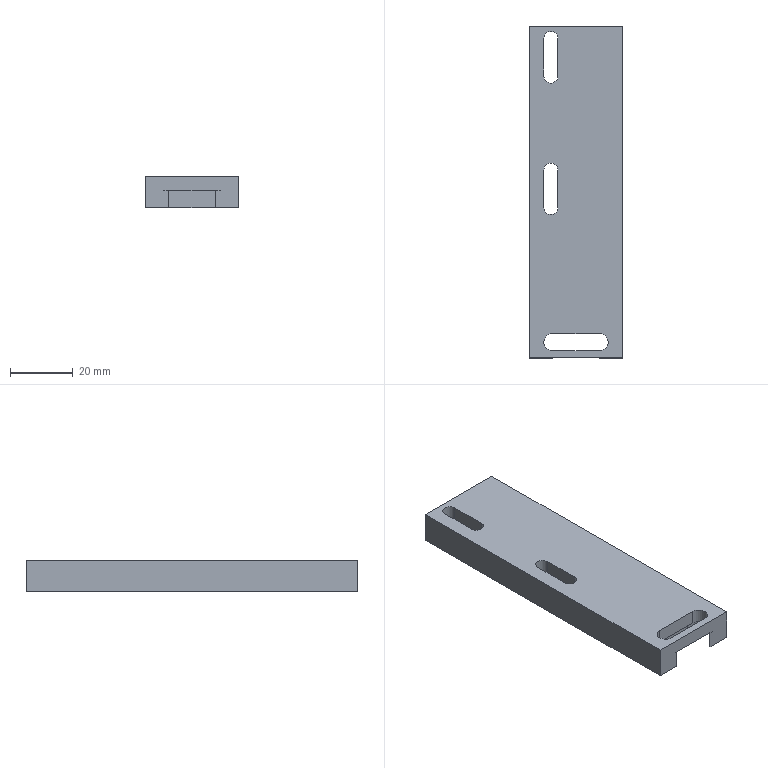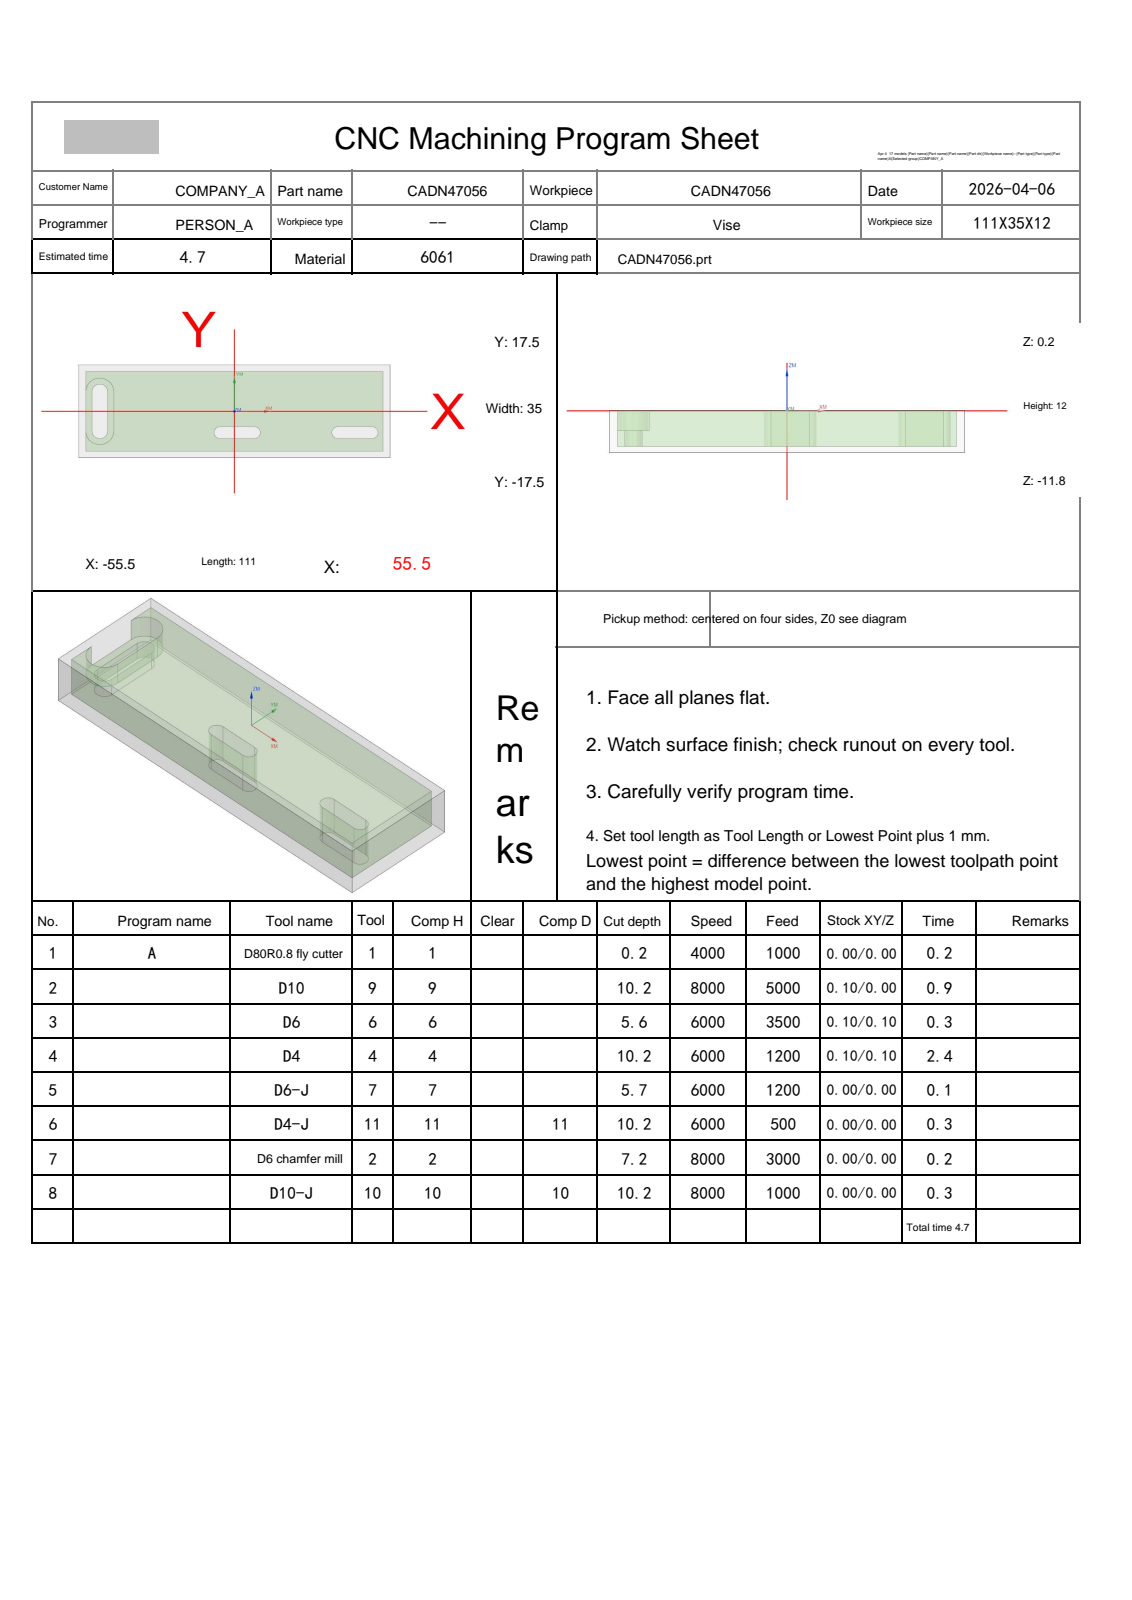NC program | NX | posted by the shop | part box 30 x 106 x 10 mm
Whole program:
%
O0001
(Machine time: 6.39 MIN)
(===Total Tool:8===)
(T1=D80R0.8 fly cutter D=80.  R=0.8  D-  H01 Z=0.    )
(T9=D10     D=10.  R=0.   D-  H09 Z=-10.  )
(T6=D6      D=6.   R=0.   D-  H06 Z=-5.4  )
(T4=D4      D=4.   R=0.   D-  H04 Z=-10.  )
(T7=D6-J    D=6.   R=0.   D7  H07 Z=-5.5  )
(T11=D4-J   D=4.   R=0.   D11 H11 Z=-10.  )
(T2=D6 chamfer mill   D=6.   R=0.   D-  H02 Z=-7.   )
(T10=D10-J  D=10.  R=0.   D10 H10 Z=-10.  )
G80 G90 G17 G49 G40
G91 G28 Z0
M01
N1 T01 M06
(D80R0.8 fly cutter  D=80. R=0.8 H=01 ce=0.00 di=0.00)
G00 G90 G54 X-98. Y0.0 M03 S4000
G43 H01 Z20.
M08
Z2.
G01 Z0.0 F1000.
X-93.
X93.
X98.
Z2.
G00 Z20.
G91 G28 Z0.0
M05
M09
G91 G28 Z0.0
M01
N2 T09 M06
(D10  D=10. R=0. H=09 ce=0.10 di=0.00)
G00 G90 G54 X0.0 Y20.1 M03 S8000
G43 H09 Z20.
M08
Z.5
G01 X53. Z.369 F5000.
G02 X58.1 Y15. Z.35 I0.0 J-5.1
G01 Y-15. Z.275
G02 X53. Y-20.1 Z.256 I-5.1 J0.0
G01 X-53. Z-.006
G02 X-58.1 Y-15. Z-.025 I0.0 J5.1
G01 Y15. Z-.1
G02 X-53. Y20.1 Z-.119 I5.1 J0.0
G01 X53. Z-.381
G02 X58.1 Y15. Z-.4 I0.0 J-5.1
G01 Y-15. Z-.475
G02 X53. Y-20.1 Z-.494 I-5.1 J0.0
G01 X-53. Z-.756
G02 X-58.1 Y-15. Z-.775 I0.0 J5.1
G01 Y15. Z-.85
G02 X-53. Y20.1 Z-.869 I5.1 J0.0
G01 X53. Z-1.131
G02 X58.1 Y15. Z-1.15 I0.0 J-5.1
G01 Y-15. Z-1.225
G02 X53. Y-20.1 Z-1.244 I-5.1 J0.0
G01 X-53. Z-1.506
G02 X-58.1 Y-15. Z-1.525 I0.0 J5.1
G01 Y15. Z-1.6
G02 X-53. Y20.1 Z-1.619 I5.1 J0.0
G01 X53. Z-1.881
G02 X58.1 Y15. Z-1.9 I0.0 J-5.1
G01 Y-15. Z-1.975
G02 X53. Y-20.1 Z-1.994 I-5.1 J0.0
G01 X-53. Z-2.256
G02 X-58.1 Y-15. Z-2.275 I0.0 J5.1
G01 Y15. Z-2.35
G02 X-53. Y20.1 Z-2.369 I5.1 J0.0
G01 X53. Z-2.631
G02 X58.1 Y15. Z-2.65 I0.0 J-5.1
G01 Y-15. Z-2.725
G02 X53. Y-20.1 Z-2.744 I-5.1 J0.0
G01 X-53. Z-3.006
G02 X-58.1 Y-15. Z-3.025 I0.0 J5.1
G01 Y15. Z-3.1
G02 X-53. Y20.1 Z-3.119 I5.1 J0.0
G01 X53. Z-3.381
G02 X58.1 Y15. Z-3.4 I0.0 J-5.1
G01 Y-15. Z-3.475
G02 X53. Y-20.1 Z-3.494 I-5.1 J0.0
G01 X-53. Z-3.756
G02 X-58.1 Y-15. Z-3.775 I0.0 J5.1
G01 Y15. Z-3.85
G02 X-53. Y20.1 Z-3.869 I5.1 J0.0
G01 X53. Z-4.131
G02 X58.1 Y15. Z-4.15 I0.0 J-5.1
G01 Y-15. Z-4.225
G02 X53. Y-20.1 Z-4.244 I-5.1 J0.0
G01 X-53. Z-4.506
G02 X-58.1 Y-15. Z-4.525 I0.0 J5.1
G01 Y15. Z-4.6
G02 X-53. Y20.1 Z-4.619 I5.1 J0.0
G01 X53. Z-4.881
G02 X58.1 Y15. Z-4.9 I0.0 J-5.1
G01 Y-15. Z-4.975
G02 X53. Y-20.1 Z-4.994 I-5.1 J0.0
G01 X-53. Z-5.256
G02 X-58.1 Y-15. Z-5.275 I0.0 J5.1
G01 Y15. Z-5.35
G02 X-53. Y20.1 Z-5.369 I5.1 J0.0
G01 X53. Z-5.631
G02 X58.1 Y15. Z-5.65 I0.0 J-5.1
G01 Y-15. Z-5.725
G02 X53. Y-20.1 Z-5.744 I-5.1 J0.0
G01 X-53. Z-6.006
G02 X-58.1 Y-15. Z-6.025 I0.0 J5.1
G01 Y15. Z-6.1
G02 X-53. Y20.1 Z-6.119 I5.1 J0.0
G01 X53. Z-6.381
G02 X58.1 Y15. Z-6.4 I0.0 J-5.1
G01 Y-15. Z-6.475
G02 X53. Y-20.1 Z-6.494 I-5.1 J0.0
G01 X-53. Z-6.756
G02 X-58.1 Y-15. Z-6.775 I0.0 J5.1
G01 Y15. Z-6.85
G02 X-53. Y20.1 Z-6.869 I5.1 J0.0
G01 X53. Z-7.131
G02 X58.1 Y15. Z-7.15 I0.0 J-5.1
G01 Y-15. Z-7.225
G02 X53. Y-20.1 Z-7.244 I-5.1 J0.0
G01 X-53. Z-7.506
G02 X-58.1 Y-15. Z-7.525 I0.0 J5.1
G01 Y15. Z-7.6
G02 X-53. Y20.1 Z-7.619 I5.1 J0.0
G01 X53. Z-7.881
G02 X58.1 Y15. Z-7.9 I0.0 J-5.1
G01 Y-15. Z-7.975
G02 X53. Y-20.1 Z-7.994 I-5.1 J0.0
G01 X-53. Z-8.256
G02 X-58.1 Y-15. Z-8.275 I0.0 J5.1
G01 Y15. Z-8.35
G02 X-53. Y20.1 Z-8.369 I5.1 J0.0
G01 X53. Z-8.631
G02 X58.1 Y15. Z-8.65 I0.0 J-5.1
G01 Y-15. Z-8.725
G02 X53. Y-20.1 Z-8.744 I-5.1 J0.0
G01 X-53. Z-9.006
G02 X-58.1 Y-15. Z-9.025 I0.0 J5.1
G01 Y15. Z-9.1
G02 X-53. Y20.1 Z-9.119 I5.1 J0.0
G01 X53. Z-9.381
G02 X58.1 Y15. Z-9.4 I0.0 J-5.1
G01 Y-15. Z-9.475
G02 X53. Y-20.1 Z-9.494 I-5.1 J0.0
G01 X-53. Z-9.756
G02 X-58.1 Y-15. Z-9.775 I0.0 J5.1
G01 Y15. Z-9.85
G02 X-53. Y20.1 Z-9.869 I5.1 J0.0
G01 X0.0 Z-10.
X53.
G02 X58.1 Y15. I0.0 J-5.1
G01 Y-15.
G02 X53. Y-20.1 I-5.1 J0.0
G01 X-53.
G02 X-58.1 Y-15. I0.0 J5.1
G01 Y15.
G02 X-53. Y20.1 I5.1 J0.0
G01 X0.0
X.5
Z-9.
G00 Z20.
G91 G28 Z0.0
M05
M09
G91 G28 Z0.0
M01
N3 T06 M06
(D6  D=6. R=0. H=06 ce=0.10 di=0.10)
G00 G90 G54 X-59. Y0.0 M03 S6000
G43 H06 Z20.
M08
Z.114
G01 Z-.386 F3500.
X-50.9
Y-2.094
G02 X-48.8 Y-3.5 I-2.1 J-5.406
G01 Y3.5
G02 X-50.9 Y2.094 I-4.2 J4.
G01 Y0.0
X-53.6
Y-4.459
G02 X-53. Y-4.4 I.6 J-3.041
X-49.9 Y-7.5 I0.0 J-3.1
G03 X-48. Y-9.4 I1.9 J0.0
X-46.1 Y-7.5 I0.0 J1.9
G01 Y7.5
G03 X-48. Y9.4 I-1.9 J0.0
X-49.9 Y7.5 I0.0 J-1.9
G02 X-53. Y4.4 I-3.1 J0.0
X-53.6 Y4.459 I0.0 J3.1
G01 Y0.0
Y-.5
Z.114
G00 Z.5
X-59. Y0.0
Z-.271
G01 Z-.771
X-50.9
Y-2.094
G02 X-48.8 Y-3.5 I-2.1 J-5.406
G01 Y3.5
G02 X-50.9 Y2.094 I-4.2 J4.
G01 Y0.0
X-53.6
Y-4.459
G02 X-53. Y-4.4 I.6 J-3.041
X-49.9 Y-7.5 I0.0 J-3.1
G03 X-48. Y-9.4 I1.9 J0.0
X-46.1 Y-7.5 I0.0 J1.9
G01 Y7.5
G03 X-48. Y9.4 I-1.9 J0.0
X-49.9 Y7.5 I0.0 J-1.9
G02 X-53. Y4.4 I-3.1 J0.0
X-53.6 Y4.459 I0.0 J3.1
G01 Y0.0
Y-.5
Z-.271
G00 Z.114
X-59. Y0.0
Z-.657
G01 Z-1.157
X-50.9
Y-2.094
G02 X-48.8 Y-3.5 I-2.1 J-5.406
G01 Y3.5
G02 X-50.9 Y2.094 I-4.2 J4.
G01 Y0.0
X-53.6
Y-4.459
G02 X-53. Y-4.4 I.6 J-3.041
X-49.9 Y-7.5 I0.0 J-3.1
G03 X-48. Y-9.4 I1.9 J0.0
X-46.1 Y-7.5 I0.0 J1.9
G01 Y7.5
G03 X-48. Y9.4 I-1.9 J0.0
X-49.9 Y7.5 I0.0 J-1.9
G02 X-53. Y4.4 I-3.1 J0.0
X-53.6 Y4.459 I0.0 J3.1
G01 Y0.0
Y-.5
Z-.657
G00 Z-.271
X-59. Y0.0
Z-1.043
G01 Z-1.543
X-50.9
Y-2.094
G02 X-48.8 Y-3.5 I-2.1 J-5.406
G01 Y3.5
G02 X-50.9 Y2.094 I-4.2 J4.
G01 Y0.0
X-53.6
Y-4.459
G02 X-53. Y-4.4 I.6 J-3.041
X-49.9 Y-7.5 I0.0 J-3.1
G03 X-48. Y-9.4 I1.9 J0.0
X-46.1 Y-7.5 I0.0 J1.9
G01 Y7.5
G03 X-48. Y9.4 I-1.9 J0.0
X-49.9 Y7.5 I0.0 J-1.9
G02 X-53. Y4.4 I-3.1 J0.0
X-53.6 Y4.459 I0.0 J3.1
G01 Y0.0
Y-.5
Z-1.043
G00 Z-.657
X-59. Y0.0
Z-1.429
G01 Z-1.929
X-50.9
Y-2.094
G02 X-48.8 Y-3.5 I-2.1 J-5.406
G01 Y3.5
G02 X-50.9 Y2.094 I-4.2 J4.
G01 Y0.0
X-53.6
Y-4.459
G02 X-53. Y-4.4 I.6 J-3.041
X-49.9 Y-7.5 I0.0 J-3.1
G03 X-48. Y-9.4 I1.9 J0.0
X-46.1 Y-7.5 I0.0 J1.9
G01 Y7.5
G03 X-48. Y9.4 I-1.9 J0.0
X-49.9 Y7.5 I0.0 J-1.9
G02 X-53. Y4.4 I-3.1 J0.0
X-53.6 Y4.459 I0.0 J3.1
G01 Y0.0
Y-.5
Z-1.429
G00 Z-1.043
X-59. Y0.0
Z-1.814
G01 Z-2.314
X-50.9
Y-2.094
G02 X-48.8 Y-3.5 I-2.1 J-5.406
G01 Y3.5
G02 X-50.9 Y2.094 I-4.2 J4.
G01 Y0.0
X-53.6
Y-4.459
G02 X-53. Y-4.4 I.6 J-3.041
X-49.9 Y-7.5 I0.0 J-3.1
G03 X-48. Y-9.4 I1.9 J0.0
X-46.1 Y-7.5 I0.0 J1.9
G01 Y7.5
G03 X-48. Y9.4 I-1.9 J0.0
X-49.9 Y7.5 I0.0 J-1.9
G02 X-53. Y4.4 I-3.1 J0.0
X-53.6 Y4.459 I0.0 J3.1
G01 Y0.0
Y-.5
Z-1.814
G00 Z-1.429
X-59. Y0.0
Z-2.2
G01 Z-2.7
X-50.9
Y-2.094
G02 X-48.8 Y-3.5 I-2.1 J-5.406
G01 Y3.5
G02 X-50.9 Y2.094 I-4.2 J4.
G01 Y0.0
X-53.6
Y-4.459
G02 X-53. Y-4.4 I.6 J-3.041
X-49.9 Y-7.5 I0.0 J-3.1
G03 X-48. Y-9.4 I1.9 J0.0
X-46.1 Y-7.5 I0.0 J1.9
G01 Y7.5
G03 X-48. Y9.4 I-1.9 J0.0
X-49.9 Y7.5 I0.0 J-1.9
G02 X-53. Y4.4 I-3.1 J0.0
X-53.6 Y4.459 I0.0 J3.1
G01 Y0.0
Y-.5
Z-2.2
G00 Z-1.814
X-59. Y0.0
Z-2.586
G01 Z-3.086
X-50.9
Y-2.094
G02 X-48.8 Y-3.5 I-2.1 J-5.406
G01 Y3.5
G02 X-50.9 Y2.094 I-4.2 J4.
G01 Y0.0
X-53.6
Y-4.459
G02 X-53. Y-4.4 I.6 J-3.041
X-49.9 Y-7.5 I0.0 J-3.1
G03 X-48. Y-9.4 I1.9 J0.0
X-46.1 Y-7.5 I0.0 J1.9
G01 Y7.5
G03 X-48. Y9.4 I-1.9 J0.0
X-49.9 Y7.5 I0.0 J-1.9
G02 X-53. Y4.4 I-3.1 J0.0
X-53.6 Y4.459 I0.0 J3.1
G01 Y0.0
Y-.5
Z-2.586
G00 Z-2.2
X-59. Y0.0
Z-2.971
G01 Z-3.471
X-50.9
Y-2.094
G02 X-48.8 Y-3.5 I-2.1 J-5.406
G01 Y3.5
G02 X-50.9 Y2.094 I-4.2 J4.
G01 Y0.0
X-53.6
Y-4.459
G02 X-53. Y-4.4 I.6 J-3.041
X-49.9 Y-7.5 I0.0 J-3.1
G03 X-48. Y-9.4 I1.9 J0.0
X-46.1 Y-7.5 I0.0 J1.9
G01 Y7.5
G03 X-48. Y9.4 I-1.9 J0.0
X-49.9 Y7.5 I0.0 J-1.9
G02 X-53. Y4.4 I-3.1 J0.0
X-53.6 Y4.459 I0.0 J3.1
G01 Y0.0
Y-.5
Z-2.971
G00 Z-2.586
X-59. Y0.0
Z-3.357
G01 Z-3.857
X-50.9
Y-2.094
G02 X-48.8 Y-3.5 I-2.1 J-5.406
G01 Y3.5
G02 X-50.9 Y2.094 I-4.2 J4.
G01 Y0.0
X-53.6
Y-4.459
G02 X-53. Y-4.4 I.6 J-3.041
X-49.9 Y-7.5 I0.0 J-3.1
G03 X-48. Y-9.4 I1.9 J0.0
X-46.1 Y-7.5 I0.0 J1.9
G01 Y7.5
G03 X-48. Y9.4 I-1.9 J0.0
X-49.9 Y7.5 I0.0 J-1.9
G02 X-53. Y4.4 I-3.1 J0.0
X-53.6 Y4.459 I0.0 J3.1
G01 Y0.0
Y-.5
Z-3.357
G00 Z-2.971
X-59. Y0.0
Z-3.743
G01 Z-4.243
X-50.9
Y-2.094
G02 X-48.8 Y-3.5 I-2.1 J-5.406
G01 Y3.5
G02 X-50.9 Y2.094 I-4.2 J4.
G01 Y0.0
X-53.6
Y-4.459
G02 X-53. Y-4.4 I.6 J-3.041
X-49.9 Y-7.5 I0.0 J-3.1
G03 X-48. Y-9.4 I1.9 J0.0
X-46.1 Y-7.5 I0.0 J1.9
G01 Y7.5
G03 X-48. Y9.4 I-1.9 J0.0
X-49.9 Y7.5 I0.0 J-1.9
G02 X-53. Y4.4 I-3.1 J0.0
X-53.6 Y4.459 I0.0 J3.1
G01 Y0.0
Y-.5
Z-3.743
G00 Z-3.357
X-59. Y0.0
Z-4.129
G01 Z-4.629
X-50.9
Y-2.094
G02 X-48.8 Y-3.5 I-2.1 J-5.406
G01 Y3.5
G02 X-50.9 Y2.094 I-4.2 J4.
G01 Y0.0
X-53.6
Y-4.459
G02 X-53. Y-4.4 I.6 J-3.041
X-49.9 Y-7.5 I0.0 J-3.1
G03 X-48. Y-9.4 I1.9 J0.0
X-46.1 Y-7.5 I0.0 J1.9
G01 Y7.5
G03 X-48. Y9.4 I-1.9 J0.0
X-49.9 Y7.5 I0.0 J-1.9
G02 X-53. Y4.4 I-3.1 J0.0
X-53.6 Y4.459 I0.0 J3.1
G01 Y0.0
Y-.5
Z-4.129
G00 Z-3.743
X-59. Y0.0
Z-4.514
G01 Z-5.014
X-50.9
Y-2.094
G02 X-48.8 Y-3.5 I-2.1 J-5.406
G01 Y3.5
G02 X-50.9 Y2.094 I-4.2 J4.
G01 Y0.0
X-53.6
Y-4.459
G02 X-53. Y-4.4 I.6 J-3.041
X-49.9 Y-7.5 I0.0 J-3.1
G03 X-48. Y-9.4 I1.9 J0.0
X-46.1 Y-7.5 I0.0 J1.9
G01 Y7.5
G03 X-48. Y9.4 I-1.9 J0.0
X-49.9 Y7.5 I0.0 J-1.9
G02 X-53. Y4.4 I-3.1 J0.0
X-53.6 Y4.459 I0.0 J3.1
G01 Y0.0
Y-.5
Z-4.514
G00 Z-4.129
X-59. Y0.0
Z-4.9
G01 Z-5.4
X-50.9
Y-2.094
G02 X-48.8 Y-3.5 I-2.1 J-5.406
G01 Y3.5
G02 X-50.9 Y2.094 I-4.2 J4.
G01 Y0.0
X-53.6
Y-4.459
G02 X-53. Y-4.4 I.6 J-3.041
X-49.9 Y-7.5 I0.0 J-3.1
G03 X-48. Y-9.4 I1.9 J0.0
X-46.1 Y-7.5 I0.0 J1.9
G01 Y7.5
G03 X-48. Y9.4 I-1.9 J0.0
X-49.9 Y7.5 I0.0 J-1.9
G02 X-53. Y4.4 I-3.1 J0.0
X-53.6 Y4.459 I0.0 J3.1
G01 Y0.0
Y-.5
Z-4.9
G00 Z20.
G91 G28 Z0.0
M05
M09
G91 G28 Z0.0
M01
N4 T04 M06
(D4  D=4. R=0. H=04 ce=0.10 di=0.10)
G00 G90 G54 X43. Y-7.85 M03 S6000
G43 H04 Z20.
M08
Z.5
G01 X37. Z.44 F1200.
G03 X36.85 Y-8. Z.438 I0.0 J-.15
X37. Y-8.15 Z.435 I.15 J0.0
G01 X49. Z.315
G03 X49.15 Y-8. Z.313 I0.0 J.15
X49. Y-7.85 Z.31 I-.15 J0.0
G01 X37. Z.19
G03 X36.85 Y-8. Z.188 I0.0 J-.15
X37. Y-8.15 Z.185 I.15 J0.0
G01 X49. Z.065
G03 X49.15 Y-8. Z.063 I0.0 J.15
X49. Y-7.85 Z.06 I-.15 J0.0
G01 X37. Z-.06
G03 X36.85 Y-8. Z-.063 I0.0 J-.15
X37. Y-8.15 Z-.065 I.15 J0.0
G01 X49. Z-.185
G03 X49.15 Y-8. Z-.188 I0.0 J.15
X49. Y-7.85 Z-.19 I-.15 J0.0
G01 X37. Z-.31
G03 X36.85 Y-8. Z-.313 I0.0 J-.15
X37. Y-8.15 Z-.315 I.15 J0.0
G01 X49. Z-.435
G03 X49.15 Y-8. Z-.438 I0.0 J.15
X49. Y-7.85 Z-.44 I-.15 J0.0
G01 X37. Z-.56
G03 X36.85 Y-8. Z-.563 I0.0 J-.15
X37. Y-8.15 Z-.565 I.15 J0.0
G01 X49. Z-.685
G03 X49.15 Y-8. Z-.688 I0.0 J.15
X49. Y-7.85 Z-.69 I-.15 J0.0
G01 X37. Z-.81
G03 X36.85 Y-8. Z-.813 I0.0 J-.15
X37. Y-8.15 Z-.815 I.15 J0.0
G01 X49. Z-.935
G03 X49.15 Y-8. Z-.938 I0.0 J.15
X49. Y-7.85 Z-.94 I-.15 J0.0
G01 X37. Z-1.06
G03 X36.85 Y-8. Z-1.063 I0.0 J-.15
X37. Y-8.15 Z-1.065 I.15 J0.0
G01 X49. Z-1.185
G03 X49.15 Y-8. Z-1.188 I0.0 J.15
X49. Y-7.85 Z-1.19 I-.15 J0.0
G01 X37. Z-1.31
G03 X36.85 Y-8. Z-1.313 I0.0 J-.15
X37. Y-8.15 Z-1.315 I.15 J0.0
G01 X49. Z-1.435
G03 X49.15 Y-8. Z-1.438 I0.0 J.15
X49. Y-7.85 Z-1.44 I-.15 J0.0
G01 X37. Z-1.56
G03 X36.85 Y-8. Z-1.563 I0.0 J-.15
X37. Y-8.15 Z-1.565 I.15 J0.0
G01 X49. Z-1.685
G03 X49.15 Y-8. Z-1.688 I0.0 J.15
X49. Y-7.85 Z-1.69 I-.15 J0.0
G01 X37. Z-1.81
G03 X36.85 Y-8. Z-1.813 I0.0 J-.15
X37. Y-8.15 Z-1.815 I.15 J0.0
G01 X49. Z-1.935
G03 X49.15 Y-8. Z-1.938 I0.0 J.15
X49. Y-7.85 Z-1.94 I-.15 J0.0
G01 X37. Z-2.06
G03 X36.85 Y-8. Z-2.063 I0.0 J-.15
X37. Y-8.15 Z-2.065 I.15 J0.0
G01 X49. Z-2.185
G03 X49.15 Y-8. Z-2.188 I0.0 J.15
X49. Y-7.85 Z-2.19 I-.15 J0.0
G01 X37. Z-2.31
G03 X36.85 Y-8. Z-2.313 I0.0 J-.15
X37. Y-8.15 Z-2.315 I.15 J0.0
G01 X49. Z-2.435
G03 X49.15 Y-8. Z-2.438 I0.0 J.15
X49. Y-7.85 Z-2.44 I-.15 J0.0
G01 X37. Z-2.56
G03 X36.85 Y-8. Z-2.563 I0.0 J-.15
X37. Y-8.15 Z-2.565 I.15 J0.0
G01 X49. Z-2.685
G03 X49.15 Y-8. Z-2.688 I0.0 J.15
X49. Y-7.85 Z-2.69 I-.15 J0.0
G01 X37. Z-2.81
G03 X36.85 Y-8. Z-2.813 I0.0 J-.15
X37. Y-8.15 Z-2.815 I.15 J0.0
G01 X49. Z-2.935
G03 X49.15 Y-8. Z-2.938 I0.0 J.15
X49. Y-7.85 Z-2.94 I-.15 J0.0
G01 X37. Z-3.06
G03 X36.85 Y-8. Z-3.063 I0.0 J-.15
X37. Y-8.15 Z-3.065 I.15 J0.0
G01 X49. Z-3.185
G03 X49.15 Y-8. Z-3.188 I0.0 J.15
X49. Y-7.85 Z-3.19 I-.15 J0.0
G01 X37. Z-3.31
G03 X36.85 Y-8. Z-3.313 I0.0 J-.15
X37. Y-8.15 Z-3.315 I.15 J0.0
G01 X49. Z-3.435
G03 X49.15 Y-8. Z-3.438 I0.0 J.15
X49. Y-7.85 Z-3.44 I-.15 J0.0
G01 X37. Z-3.56
G03 X36.85 Y-8. Z-3.563 I0.0 J-.15
X37. Y-8.15 Z-3.565 I.15 J0.0
G01 X49. Z-3.685
G03 X49.15 Y-8. Z-3.688 I0.0 J.15
X49. Y-7.85 Z-3.69 I-.15 J0.0
G01 X37. Z-3.81
G03 X36.85 Y-8. Z-3.813 I0.0 J-.15
X37. Y-8.15 Z-3.815 I.15 J0.0
G01 X49. Z-3.935
G03 X49.15 Y-8. Z-3.938 I0.0 J.15
X49. Y-7.85 Z-3.94 I-.15 J0.0
G01 X37. Z-4.06
G03 X36.85 Y-8. Z-4.063 I0.0 J-.15
X37. Y-8.15 Z-4.065 I.15 J0.0
G01 X49. Z-4.185
G03 X49.15 Y-8. Z-4.188 I0.0 J.15
X49. Y-7.85 Z-4.19 I-.15 J0.0
G01 X37. Z-4.31
G03 X36.85 Y-8. Z-4.313 I0.0 J-.15
X37. Y-8.15 Z-4.315 I.15 J0.0
G01 X49. Z-4.435
G03 X49.15 Y-8. Z-4.438 I0.0 J.15
X49. Y-7.85 Z-4.44 I-.15 J0.0
G01 X37. Z-4.56
G03 X36.85 Y-8. Z-4.563 I0.0 J-.15
X37. Y-8.15 Z-4.565 I.15 J0.0
G01 X49. Z-4.685
G03 X49.15 Y-8. Z-4.688 I0.0 J.15
X49. Y-7.85 Z-4.69 I-.15 J0.0
G01 X37. Z-4.81
G03 X36.85 Y-8. Z-4.813 I0.0 J-.15
X37. Y-8.15 Z-4.815 I.15 J0.0
G01 X49. Z-4.935
G03 X49.15 Y-8. Z-4.938 I0.0 J.15
X49. Y-7.85 Z-4.94 I-.15 J0.0
G01 X37. Z-5.06
G03 X36.85 Y-8. Z-5.063 I0.0 J-.15
X37. Y-8.15 Z-5.065 I.15 J0.0
G01 X49. Z-5.185
G03 X49.15 Y-8. Z-5.188 I0.0 J.15
X49. Y-7.85 Z-5.19 I-.15 J0.0
G01 X37. Z-5.31
G03 X36.85 Y-8. Z-5.313 I0.0 J-.15
X37. Y-8.15 Z-5.315 I.15 J0.0
G01 X49. Z-5.435
G03 X49.15 Y-8. Z-5.438 I0.0 J.15
X49. Y-7.85 Z-5.44 I-.15 J0.0
G01 X37. Z-5.56
G03 X36.85 Y-8. Z-5.563 I0.0 J-.15
X37. Y-8.15 Z-5.565 I.15 J0.0
G01 X49. Z-5.685
G03 X49.15 Y-8. Z-5.688 I0.0 J.15
X49. Y-7.85 Z-5.69 I-.15 J0.0
G01 X37. Z-5.81
G03 X36.85 Y-8. Z-5.813 I0.0 J-.15
X37. Y-8.15 Z-5.815 I.15 J0.0
G01 X49. Z-5.935
G03 X49.15 Y-8. Z-5.938 I0.0 J.15
X49. Y-7.85 Z-5.94 I-.15 J0.0
G01 X37. Z-6.06
G03 X36.85 Y-8. Z-6.063 I0.0 J-.15
X37. Y-8.15 Z-6.065 I.15 J0.0
G01 X49. Z-6.185
G03 X49.15 Y-8. Z-6.188 I0.0 J.15
X49. Y-7.85 Z-6.19 I-.15 J0.0
G01 X37. Z-6.31
G03 X36.85 Y-8. Z-6.313 I0.0 J-.15
X37. Y-8.15 Z-6.315 I.15 J0.0
G01 X49. Z-6.435
G03 X49.15 Y-8. Z-6.438 I0.0 J.15
X49. Y-7.85 Z-6.44 I-.15 J0.0
G01 X37. Z-6.56
G03 X36.85 Y-8. Z-6.563 I0.0 J-.15
X37. Y-8.15 Z-6.565 I.15 J0.0
G01 X49. Z-6.685
G03 X49.15 Y-8. Z-6.688 I0.0 J.15
X49. Y-7.85 Z-6.69 I-.15 J0.0
G01 X37. Z-6.81
G03 X36.85 Y-8. Z-6.813 I0.0 J-.15
X37. Y-8.15 Z-6.815 I.15 J0.0
G01 X49. Z-6.935
G03 X49.15 Y-8. Z-6.938 I0.0 J.15
X49. Y-7.85 Z-6.94 I-.15 J0.0
G01 X37. Z-7.06
G03 X36.85 Y-8. Z-7.063 I0.0 J-.15
X37. Y-8.15 Z-7.065 I.15 J0.0
G01 X49. Z-7.185
G03 X49.15 Y-8. Z-7.188 I0.0 J.15
X49. Y-7.85 Z-7.19 I-.15 J0.0
G01 X37. Z-7.31
G03 X36.85 Y-8. Z-7.313 I0.0 J-.15
X37. Y-8.15 Z-7.315 I.15 J0.0
G01 X49. Z-7.435
G03 X49.15 Y-8. Z-7.438 I0.0 J.15
X49. Y-7.85 Z-7.44 I-.15 J0.0
G01 X37. Z-7.56
G03 X36.85 Y-8. Z-7.563 I0.0 J-.15
X37. Y-8.15 Z-7.565 I.15 J0.0
G01 X49. Z-7.685
G03 X49.15 Y-8. Z-7.688 I0.0 J.15
X49. Y-7.85 Z-7.69 I-.15 J0.0
G01 X37. Z-7.81
G03 X36.85 Y-8. Z-7.813 I0.0 J-.15
X37. Y-8.15 Z-7.815 I.15 J0.0
G01 X49. Z-7.935
G03 X49.15 Y-8. Z-7.938 I0.0 J.15
X49. Y-7.85 Z-7.94 I-.15 J0.0
G01 X37. Z-8.06
G03 X36.85 Y-8. Z-8.063 I0.0 J-.15
X37. Y-8.15 Z-8.065 I.15 J0.0
G01 X49. Z-8.185
G03 X49.15 Y-8. Z-8.188 I0.0 J.15
X49. Y-7.85 Z-8.19 I-.15 J0.0
G01 X37. Z-8.31
G03 X36.85 Y-8. Z-8.313 I0.0 J-.15
X37. Y-8.15 Z-8.315 I.15 J0.0
G01 X49. Z-8.435
G03 X49.15 Y-8. Z-8.438 I0.0 J.15
X49. Y-7.85 Z-8.44 I-.15 J0.0
G01 X37. Z-8.56
G03 X36.85 Y-8. Z-8.563 I0.0 J-.15
X37. Y-8.15 Z-8.565 I.15 J0.0
G01 X49. Z-8.685
G03 X49.15 Y-8. Z-8.688 I0.0 J.15
X49. Y-7.85 Z-8.69 I-.15 J0.0
G01 X37. Z-8.81
G03 X36.85 Y-8. Z-8.813 I0.0 J-.15
X37. Y-8.15 Z-8.815 I.15 J0.0
G01 X49. Z-8.935
G03 X49.15 Y-8. Z-8.938 I0.0 J.15
X49. Y-7.85 Z-8.94 I-.15 J0.0
G01 X37. Z-9.06
G03 X36.85 Y-8. Z-9.063 I0.0 J-.15
X37. Y-8.15 Z-9.065 I.15 J0.0
G01 X49. Z-9.185
G03 X49.15 Y-8. Z-9.188 I0.0 J.15
X49. Y-7.85 Z-9.19 I-.15 J0.0
G01 X37. Z-9.31
G03 X36.85 Y-8. Z-9.313 I0.0 J-.15
X37. Y-8.15 Z-9.315 I.15 J0.0
G01 X49. Z-9.435
G03 X49.15 Y-8. Z-9.438 I0.0 J.15
X49. Y-7.85 Z-9.44 I-.15 J0.0
G01 X37. Z-9.56
G03 X36.85 Y-8. Z-9.563 I0.0 J-.15
X37. Y-8.15 Z-9.565 I.15 J0.0
G01 X49. Z-9.685
G03 X49.15 Y-8. Z-9.688 I0.0 J.15
X49. Y-7.85 Z-9.69 I-.15 J0.0
G01 X37. Z-9.81
G03 X36.85 Y-8. Z-9.813 I0.0 J-.15
X37. Y-8.15 Z-9.815 I.15 J0.0
G01 X49. Z-9.935
G03 X49.15 Y-8. Z-9.938 I0.0 J.15
X49. Y-7.85 Z-9.94 I-.15 J0.0
G01 X43. Z-10.
X37.
G03 X36.85 Y-8. I0.0 J-.15
X37. Y-8.15 I.15 J0.0
G01 X49.
G03 X49.15 Y-8. I0.0 J.15
X49. Y-7.85 I-.15 J0.0
G01 X43.
X42.5
Z-9.
G00 Z20.
X1.
Z.5
G01 X-5. Z.44
G03 X-5.15 Y-8. Z.438 I0.0 J-.15
X-5. Y-8.15 Z.435 I.15 J0.0
G01 X7. Z.315
G03 X7.15 Y-8. Z.313 I0.0 J.15
X7. Y-7.85 Z.31 I-.15 J0.0
G01 X-5. Z.19
G03 X-5.15 Y-8. Z.188 I0.0 J-.15
X-5. Y-8.15 Z.185 I.15 J0.0
G01 X7. Z.065
G03 X7.15 Y-8. Z.063 I0.0 J.15
X7. Y-7.85 Z.06 I-.15 J0.0
G01 X-5. Z-.06
G03 X-5.15 Y-8. Z-.063 I0.0 J-.15
X-5. Y-8.15 Z-.065 I.15 J0.0
G01 X7. Z-.185
G03 X7.15 Y-8. Z-.188 I0.0 J.15
X7. Y-7.85 Z-.19 I-.15 J0.0
G01 X-5. Z-.31
G03 X-5.15 Y-8. Z-.313 I0.0 J-.15
X-5. Y-8.15 Z-.315 I.15 J0.0
G01 X7. Z-.435
G03 X7.15 Y-8. Z-.438 I0.0 J.15
X7. Y-7.85 Z-.44 I-.15 J0.0
G01 X-5. Z-.56
G03 X-5.15 Y-8. Z-.563 I0.0 J-.15
X-5. Y-8.15 Z-.565 I.15 J0.0
G01 X7. Z-.685
G03 X7.15 Y-8. Z-.688 I0.0 J.15
X7. Y-7.85 Z-.69 I-.15 J0.0
G01 X-5. Z-.81
G03 X-5.15 Y-8. Z-.813 I0.0 J-.15
X-5. Y-8.15 Z-.815 I.15 J0.0
G01 X7. Z-.935
G03 X7.15 Y-8. Z-.938 I0.0 J.15
X7. Y-7.85 Z-.94 I-.15 J0.0
G01 X-5. Z-1.06
G03 X-5.15 Y-8. Z-1.063 I0.0 J-.15
X-5. Y-8.15 Z-1.065 I.15 J0.0
G01 X7. Z-1.185
G03 X7.15 Y-8. Z-1.188 I0.0 J.15
X7. Y-7.85 Z-1.19 I-.15 J0.0
G01 X-5. Z-1.31
G03 X-5.15 Y-8. Z-1.313 I0.0 J-.15
X-5. Y-8.15 Z-1.315 I.15 J0.0
G01 X7. Z-1.435
G03 X7.15 Y-8. Z-1.438 I0.0 J.15
X7. Y-7.85 Z-1.44 I-.15 J0.0
G01 X-5. Z-1.56
G03 X-5.15 Y-8. Z-1.563 I0.0 J-.15
X-5. Y-8.15 Z-1.565 I.15 J0.0
G01 X7. Z-1.685
G03 X7.15 Y-8. Z-1.688 I0.0 J.15
X7. Y-7.85 Z-1.69 I-.15 J0.0
G01 X-5. Z-1.81
G03 X-5.15 Y-8. Z-1.813 I0.0 J-.15
X-5. Y-8.15 Z-1.815 I.15 J0.0
G01 X7. Z-1.935
G03 X7.15 Y-8. Z-1.938 I0.0 J.15
X7. Y-7.85 Z-1.94 I-.15 J0.0
G01 X-5. Z-2.06
G03 X-5.15 Y-8. Z-2.063 I0.0 J-.15
X-5. Y-8.15 Z-2.065 I.15 J0.0
G01 X7. Z-2.185
G03 X7.15 Y-8. Z-2.188 I0.0 J.15
X7. Y-7.85 Z-2.19 I-.15 J0.0
G01 X-5. Z-2.31
G03 X-5.15 Y-8. Z-2.313 I0.0 J-.15
X-5. Y-8.15 Z-2.315 I.15 J0.0
G01 X7. Z-2.435
G03 X7.15 Y-8. Z-2.438 I0.0 J.15
X7. Y-7.85 Z-2.44 I-.15 J0.0
G01 X-5. Z-2.56
G03 X-5.15 Y-8. Z-2.563 I0.0 J-.15
X-5. Y-8.15 Z-2.565 I.15 J0.0
G01 X7. Z-2.685
G03 X7.15 Y-8. Z-2.688 I0.0 J.15
X7. Y-7.85 Z-2.69 I-.15 J0.0
G01 X-5. Z-2.81
G03 X-5.15 Y-8. Z-2.813 I0.0 J-.15
X-5. Y-8.15 Z-2.815 I.15 J0.0
G01 X7. Z-2.935
G03 X7.15 Y-8. Z-2.938 I0.0 J.15
X7. Y-7.85 Z-2.94 I-.15 J0.0
G01 X-5. Z-3.06
G03 X-5.15 Y-8. Z-3.063 I0.0 J-.15
X-5. Y-8.15 Z-3.065 I.15 J0.0
G01 X7. Z-3.185
G03 X7.15 Y-8. Z-3.188 I0.0 J.15
X7. Y-7.85 Z-3.19 I-.15 J0.0
G01 X-5. Z-3.31
G03 X-5.15 Y-8. Z-3.313 I0.0 J-.15
X-5. Y-8.15 Z-3.315 I.15 J0.0
G01 X7. Z-3.435
G03 X7.15 Y-8. Z-3.438 I0.0 J.15
X7. Y-7.85 Z-3.44 I-.15 J0.0
G01 X-5. Z-3.56
G03 X-5.15 Y-8. Z-3.563 I0.0 J-.15
X-5. Y-8.15 Z-3.565 I.15 J0.0
G01 X7. Z-3.685
G03 X7.15 Y-8. Z-3.688 I0.0 J.15
X7. Y-7.85 Z-3.69 I-.15 J0.0
G01 X-5. Z-3.81
G03 X-5.15 Y-8. Z-3.813 I0.0 J-.15
X-5. Y-8.15 Z-3.815 I.15 J0.0
G01 X7. Z-3.935
G03 X7.15 Y-8. Z-3.938 I0.0 J.15
X7. Y-7.85 Z-3.94 I-.15 J0.0
G01 X-5. Z-4.06
G03 X-5.15 Y-8. Z-4.063 I0.0 J-.15
X-5. Y-8.15 Z-4.065 I.15 J0.0
G01 X7. Z-4.185
G03 X7.15 Y-8. Z-4.188 I0.0 J.15
X7. Y-7.85 Z-4.19 I-.15 J0.0
G01 X-5. Z-4.31
G03 X-5.15 Y-8. Z-4.313 I0.0 J-.15
X-5. Y-8.15 Z-4.315 I.15 J0.0
G01 X7. Z-4.435
G03 X7.15 Y-8. Z-4.438 I0.0 J.15
X7. Y-7.85 Z-4.44 I-.15 J0.0
G01 X-5. Z-4.56
G03 X-5.15 Y-8. Z-4.563 I0.0 J-.15
X-5. Y-8.15 Z-4.565 I.15 J0.0
G01 X7. Z-4.685
G03 X7.15 Y-8. Z-4.688 I0.0 J.15
X7. Y-7.85 Z-4.69 I-.15 J0.0
G01 X-5. Z-4.81
G03 X-5.15 Y-8. Z-4.813 I0.0 J-.15
X-5. Y-8.15 Z-4.815 I.15 J0.0
G01 X7. Z-4.935
G03 X7.15 Y-8. Z-4.938 I0.0 J.15
X7. Y-7.85 Z-4.94 I-.15 J0.0
G01 X-5. Z-5.06
G03 X-5.15 Y-8. Z-5.063 I0.0 J-.15
X-5. Y-8.15 Z-5.065 I.15 J0.0
G01 X7. Z-5.185
G03 X7.15 Y-8. Z-5.188 I0.0 J.15
X7. Y-7.85 Z-5.19 I-.15 J0.0
G01 X-5. Z-5.31
G03 X-5.15 Y-8. Z-5.313 I0.0 J-.15
X-5. Y-8.15 Z-5.315 I.15 J0.0
G01 X7. Z-5.435
G03 X7.15 Y-8. Z-5.438 I0.0 J.15
X7. Y-7.85 Z-5.44 I-.15 J0.0
G01 X-5. Z-5.56
G03 X-5.15 Y-8. Z-5.563 I0.0 J-.15
X-5. Y-8.15 Z-5.565 I.15 J0.0
G01 X7. Z-5.685
G03 X7.15 Y-8. Z-5.688 I0.0 J.15
X7. Y-7.85 Z-5.69 I-.15 J0.0
G01 X-5. Z-5.81
G03 X-5.15 Y-8. Z-5.813 I0.0 J-.15
X-5. Y-8.15 Z-5.815 I.15 J0.0
G01 X7. Z-5.935
G03 X7.15 Y-8. Z-5.938 I0.0 J.15
X7. Y-7.85 Z-5.94 I-.15 J0.0
G01 X-5. Z-6.06
G03 X-5.15 Y-8. Z-6.063 I0.0 J-.15
X-5. Y-8.15 Z-6.065 I.15 J0.0
G01 X7. Z-6.185
G03 X7.15 Y-8. Z-6.188 I0.0 J.15
X7. Y-7.85 Z-6.19 I-.15 J0.0
G01 X-5. Z-6.31
G03 X-5.15 Y-8. Z-6.313 I0.0 J-.15
X-5. Y-8.15 Z-6.315 I.15 J0.0
G01 X7. Z-6.435
G03 X7.15 Y-8. Z-6.438 I0.0 J.15
X7. Y-7.85 Z-6.44 I-.15 J0.0
G01 X-5. Z-6.56
G03 X-5.15 Y-8. Z-6.563 I0.0 J-.15
X-5. Y-8.15 Z-6.565 I.15 J0.0
G01 X7. Z-6.685
G03 X7.15 Y-8. Z-6.688 I0.0 J.15
X7. Y-7.85 Z-6.69 I-.15 J0.0
G01 X-5. Z-6.81
G03 X-5.15 Y-8. Z-6.813 I0.0 J-.15
X-5. Y-8.15 Z-6.815 I.15 J0.0
G01 X7. Z-6.935
G03 X7.15 Y-8. Z-6.938 I0.0 J.15
X7. Y-7.85 Z-6.94 I-.15 J0.0
G01 X-5. Z-7.06
G03 X-5.15 Y-8. Z-7.063 I0.0 J-.15
X-5. Y-8.15 Z-7.065 I.15 J0.0
G01 X7. Z-7.185
G03 X7.15 Y-8. Z-7.188 I0.0 J.15
X7. Y-7.85 Z-7.19 I-.15 J0.0
G01 X-5. Z-7.31
G03 X-5.15 Y-8. Z-7.313 I0.0 J-.15
X-5. Y-8.15 Z-7.315 I.15 J0.0
G01 X7. Z-7.435
G03 X7.15 Y-8. Z-7.438 I0.0 J.15
X7. Y-7.85 Z-7.44 I-.15 J0.0
G01 X-5. Z-7.56
G03 X-5.15 Y-8. Z-7.563 I0.0 J-.15
X-5. Y-8.15 Z-7.565 I.15 J0.0
G01 X7. Z-7.685
G03 X7.15 Y-8. Z-7.688 I0.0 J.15
X7. Y-7.85 Z-7.69 I-.15 J0.0
G01 X-5. Z-7.81
G03 X-5.15 Y-8. Z-7.813 I0.0 J-.15
X-5. Y-8.15 Z-7.815 I.15 J0.0
G01 X7. Z-7.935
G03 X7.15 Y-8. Z-7.938 I0.0 J.15
X7. Y-7.85 Z-7.94 I-.15 J0.0
G01 X-5. Z-8.06
G03 X-5.15 Y-8. Z-8.063 I0.0 J-.15
X-5. Y-8.15 Z-8.065 I.15 J0.0
G01 X7. Z-8.185
G03 X7.15 Y-8. Z-8.188 I0.0 J.15
X7. Y-7.85 Z-8.19 I-.15 J0.0
G01 X-5. Z-8.31
G03 X-5.15 Y-8. Z-8.313 I0.0 J-.15
X-5. Y-8.15 Z-8.315 I.15 J0.0
G01 X7. Z-8.435
G03 X7.15 Y-8. Z-8.438 I0.0 J.15
X7. Y-7.85 Z-8.44 I-.15 J0.0
G01 X-5. Z-8.56
G03 X-5.15 Y-8. Z-8.563 I0.0 J-.15
X-5. Y-8.15 Z-8.565 I.15 J0.0
G01 X7. Z-8.685
G03 X7.15 Y-8. Z-8.688 I0.0 J.15
X7. Y-7.85 Z-8.69 I-.15 J0.0
G01 X-5. Z-8.81
G03 X-5.15 Y-8. Z-8.813 I0.0 J-.15
X-5. Y-8.15 Z-8.815 I.15 J0.0
G01 X7. Z-8.935
G03 X7.15 Y-8. Z-8.938 I0.0 J.15
X7. Y-7.85 Z-8.94 I-.15 J0.0
G01 X-5. Z-9.06
G03 X-5.15 Y-8. Z-9.063 I0.0 J-.15
X-5. Y-8.15 Z-9.065 I.15 J0.0
G01 X7. Z-9.185
G03 X7.15 Y-8. Z-9.188 I0.0 J.15
X7. Y-7.85 Z-9.19 I-.15 J0.0
G01 X-5. Z-9.31
G03 X-5.15 Y-8. Z-9.313 I0.0 J-.15
X-5. Y-8.15 Z-9.315 I.15 J0.0
G01 X7. Z-9.435
G03 X7.15 Y-8. Z-9.438 I0.0 J.15
X7. Y-7.85 Z-9.44 I-.15 J0.0
G01 X-5. Z-9.56
G03 X-5.15 Y-8. Z-9.563 I0.0 J-.15
X-5. Y-8.15 Z-9.565 I.15 J0.0
G01 X7. Z-9.685
G03 X7.15 Y-8. Z-9.688 I0.0 J.15
X7. Y-7.85 Z-9.69 I-.15 J0.0
G01 X-5. Z-9.81
G03 X-5.15 Y-8. Z-9.813 I0.0 J-.15
X-5. Y-8.15 Z-9.815 I.15 J0.0
G01 X7. Z-9.935
G03 X7.15 Y-8. Z-9.938 I0.0 J.15
X7. Y-7.85 Z-9.94 I-.15 J0.0
G01 X1. Z-10.
X-5.
G03 X-5.15 Y-8. I0.0 J-.15
X-5. Y-8.15 I.15 J0.0
G01 X7.
G03 X7.15 Y-8. I0.0 J.15
X7. Y-7.85 I-.15 J0.0
G01 X1.
X.5
Z-9.
G00 Z20.
G00 G90 X-48.65 Y0.0 M03 S6000
Z20.
Z-5.
G01 Y-7.5 Z-5.055 F1200.
G03 X-48. Y-8.15 Z-5.063 I.65 J0.0
X-47.35 Y-7.5 Z-5.07 I0.0 J.65
G01 Y7.5 Z-5.18
G03 X-48. Y8.15 Z-5.188 I-.65 J0.0
X-48.65 Y7.5 Z-5.195 I0.0 J-.65
G01 Y-7.5 Z-5.305
G03 X-48. Y-8.15 Z-5.313 I.65 J0.0
X-47.35 Y-7.5 Z-5.32 I0.0 J.65
G01 Y7.5 Z-5.43
G03 X-48. Y8.15 Z-5.438 I-.65 J0.0
X-48.65 Y7.5 Z-5.445 I0.0 J-.65
G01 Y-7.5 Z-5.555
G03 X-48. Y-8.15 Z-5.563 I.65 J0.0
X-47.35 Y-7.5 Z-5.57 I0.0 J.65
G01 Y7.5 Z-5.68
G03 X-48. Y8.15 Z-5.688 I-.65 J0.0
X-48.65 Y7.5 Z-5.695 I0.0 J-.65
G01 Y-7.5 Z-5.805
G03 X-48. Y-8.15 Z-5.813 I.65 J0.0
X-47.35 Y-7.5 Z-5.82 I0.0 J.65
G01 Y7.5 Z-5.93
G03 X-48. Y8.15 Z-5.938 I-.65 J0.0
X-48.65 Y7.5 Z-5.945 I0.0 J-.65
G01 Y-7.5 Z-6.055
G03 X-48. Y-8.15 Z-6.063 I.65 J0.0
X-47.35 Y-7.5 Z-6.07 I0.0 J.65
G01 Y7.5 Z-6.18
G03 X-48. Y8.15 Z-6.188 I-.65 J0.0
X-48.65 Y7.5 Z-6.195 I0.0 J-.65
G01 Y-7.5 Z-6.305
G03 X-48. Y-8.15 Z-6.313 I.65 J0.0
X-47.35 Y-7.5 Z-6.32 I0.0 J.65
G01 Y7.5 Z-6.43
G03 X-48. Y8.15 Z-6.438 I-.65 J0.0
X-48.65 Y7.5 Z-6.445 I0.0 J-.65
G01 Y-7.5 Z-6.555
G03 X-48. Y-8.15 Z-6.563 I.65 J0.0
X-47.35 Y-7.5 Z-6.57 I0.0 J.65
G01 Y7.5 Z-6.68
G03 X-48. Y8.15 Z-6.688 I-.65 J0.0
X-48.65 Y7.5 Z-6.695 I0.0 J-.65
G01 Y-7.5 Z-6.805
G03 X-48. Y-8.15 Z-6.813 I.65 J0.0
X-47.35 Y-7.5 Z-6.82 I0.0 J.65
G01 Y7.5 Z-6.93
G03 X-48. Y8.15 Z-6.938 I-.65 J0.0
X-48.65 Y7.5 Z-6.945 I0.0 J-.65
G01 Y-7.5 Z-7.055
G03 X-48. Y-8.15 Z-7.063 I.65 J0.0
X-47.35 Y-7.5 Z-7.07 I0.0 J.65
G01 Y7.5 Z-7.18
G03 X-48. Y8.15 Z-7.188 I-.65 J0.0
X-48.65 Y7.5 Z-7.195 I0.0 J-.65
G01 Y-7.5 Z-7.305
G03 X-48. Y-8.15 Z-7.313 I.65 J0.0
X-47.35 Y-7.5 Z-7.32 I0.0 J.65
G01 Y7.5 Z-7.43
G03 X-48. Y8.15 Z-7.438 I-.65 J0.0
X-48.65 Y7.5 Z-7.445 I0.0 J-.65
G01 Y-7.5 Z-7.555
G03 X-48. Y-8.15 Z-7.563 I.65 J0.0
X-47.35 Y-7.5 Z-7.57 I0.0 J.65
G01 Y7.5 Z-7.68
G03 X-48. Y8.15 Z-7.688 I-.65 J0.0
X-48.65 Y7.5 Z-7.695 I0.0 J-.65
G01 Y-7.5 Z-7.805
G03 X-48. Y-8.15 Z-7.813 I.65 J0.0
X-47.35 Y-7.5 Z-7.82 I0.0 J.65
G01 Y7.5 Z-7.93
G03 X-48. Y8.15 Z-7.938 I-.65 J0.0
X-48.65 Y7.5 Z-7.945 I0.0 J-.65
G01 Y-7.5 Z-8.055
G03 X-48. Y-8.15 Z-8.063 I.65 J0.0
X-47.35 Y-7.5 Z-8.07 I0.0 J.65
G01 Y7.5 Z-8.18
G03 X-48. Y8.15 Z-8.188 I-.65 J0.0
X-48.65 Y7.5 Z-8.195 I0.0 J-.65
G01 Y-7.5 Z-8.305
G03 X-48. Y-8.15 Z-8.313 I.65 J0.0
X-47.35 Y-7.5 Z-8.32 I0.0 J.65
G01 Y7.5 Z-8.43
G03 X-48. Y8.15 Z-8.438 I-.65 J0.0
X-48.65 Y7.5 Z-8.445 I0.0 J-.65
G01 Y-7.5 Z-8.555
G03 X-48. Y-8.15 Z-8.563 I.65 J0.0
X-47.35 Y-7.5 Z-8.57 I0.0 J.65
G01 Y7.5 Z-8.68
G03 X-48. Y8.15 Z-8.688 I-.65 J0.0
X-48.65 Y7.5 Z-8.695 I0.0 J-.65
G01 Y-7.5 Z-8.805
G03 X-48. Y-8.15 Z-8.813 I.65 J0.0
X-47.35 Y-7.5 Z-8.82 I0.0 J.65
G01 Y7.5 Z-8.93
G03 X-48. Y8.15 Z-8.938 I-.65 J0.0
X-48.65 Y7.5 Z-8.945 I0.0 J-.65
G01 Y-7.5 Z-9.055
G03 X-48. Y-8.15 Z-9.063 I.65 J0.0
X-47.35 Y-7.5 Z-9.07 I0.0 J.65
G01 Y7.5 Z-9.18
G03 X-48. Y8.15 Z-9.188 I-.65 J0.0
X-48.65 Y7.5 Z-9.195 I0.0 J-.65
G01 Y-7.5 Z-9.305
G03 X-48. Y-8.15 Z-9.313 I.65 J0.0
X-47.35 Y-7.5 Z-9.32 I0.0 J.65
G01 Y7.5 Z-9.43
G03 X-48. Y8.15 Z-9.438 I-.65 J0.0
X-48.65 Y7.5 Z-9.445 I0.0 J-.65
G01 Y-7.5 Z-9.555
G03 X-48. Y-8.15 Z-9.563 I.65 J0.0
X-47.35 Y-7.5 Z-9.57 I0.0 J.65
G01 Y7.5 Z-9.68
G03 X-48. Y8.15 Z-9.688 I-.65 J0.0
X-48.65 Y7.5 Z-9.695 I0.0 J-.65
G01 Y-7.5 Z-9.805
G03 X-48. Y-8.15 Z-9.813 I.65 J0.0
X-47.35 Y-7.5 Z-9.82 I0.0 J.65
G01 Y7.5 Z-9.93
G03 X-48. Y8.15 Z-9.938 I-.65 J0.0
X-48.65 Y7.5 Z-9.945 I0.0 J-.65
G01 Y0.0 Z-10.
Y-7.5
G03 X-48. Y-8.15 I.65 J0.0
X-47.35 Y-7.5 I0.0 J.65
G01 Y7.5
G03 X-48. Y8.15 I-.65 J0.0
X-48.65 Y7.5 I0.0 J-.65
G01 Y0.0
Y-.5
Z-9.
G00 Z20.
G91 G28 Z0.0
M05
M09
G91 G28 Z0.0
M01
N5 T07 M06
(D6-J  D=6. R=0. H=07 ce=0.30 di=0.00)
G00 G90 G54 X-59. Y0.0 M03 S6000
G43 H07 Z20.
M08
Z-5.
G01 Z-5.5 F1200.
X-53.6
Y4.255
G03 X-53. Y4.2 I.6 J3.245
X-49.7 Y7.5 I0.0 J3.3
G02 X-48. Y9.2 I1.7 J0.0
X-46.3 Y7.5 I0.0 J-1.7
G01 Y-7.5
G02 X-48. Y-9.2 I-1.7 J0.0
X-49.7 Y-7.5 I0.0 J1.7
G03 X-53. Y-4.2 I-3.3 J0.0
X-53.6 Y-4.255 I0.0 J-3.3
G01 Y0.0
X-50.9
Y1.88
G03 X-49. Y3.028 I-2.1 J5.62
G01 Y-3.028
G03 X-50.9 Y-1.88 I-4. J-4.472
G01 Y0.0
Y.5
X-59.
Z-5.
G00 Z20.
G00 G90 X-57.021 Y-6.703 M03 S6000
Z20.
Z-4.995
G01 Z-5.495 F1200.
G41 D07
X-56.926 Y-6.734
G03 X-56.613 Y-6.784 I.313 J.95
X-55.71 Y-6.213 I0.0 J1.
G02 X-53. Y-4.5 I2.71 J-1.287
X-50. Y-7.5 I0.0 J-3.
G03 X-48. Y-9.5 I2. J0.0
X-46. Y-7.5 I0.0 J2.
G01 Y7.5
G03 X-48. Y9.5 I-2. J0.0
X-50. Y7.5 I0.0 J-2.
G02 X-53. Y4.5 I-3. J0.0
X-55.71 Y6.213 I0.0 J3.
G03 X-56.613 Y6.784 I-.903 J-.429
X-56.926 Y6.734 I0.0 J-1.
G01 G40 X-57.021 Y6.703
Z-4.995
G00 Z20.
G91 G28 Z0.0
M05
M09
G91 G28 Z0.0
M01
N6 T11 M06
(D4-J  D=4. R=0. H=11 ce=0.00 di=0.00)
G00 G90 G54 X43.2 Y-8. M03 S6000
G43 H11 Z20.
M08
Z-4.5
G01 Z-5. F500.
G41 D11
Y-7.95
G03 X43. Y-7.75 I-.2 J0.0
G01 X37.
G03 X36.75 Y-8. I0.0 J-.25
X37. Y-8.25 I.25 J0.0
G01 X49.
G03 X49.25 Y-8. I0.0 J.25
X49. Y-7.75 I-.25 J0.0
G01 X43.
X42.5
G03 X42.3 Y-7.95 I0.0 J-.2
G01 G40 Y-8.
Z-4.5
G00 Z1.
X43.2
Z-9.5
G01 Z-10.
G41 D11
Y-7.95
G03 X43. Y-7.75 I-.2 J0.0
G01 X37.
G03 X36.75 Y-8. I0.0 J-.25
X37. Y-8.25 I.25 J0.0
G01 X49.
G03 X49.25 Y-8. I0.0 J.25
X49. Y-7.75 I-.25 J0.0
G01 X43.
X42.5
G03 X42.3 Y-7.95 I0.0 J-.2
G01 G40 Y-8.
Z-9.5
G00 Z20.
X.8
Z-4.5
G01 Z-5.
G41 D11
Y-8.05
G03 X1. Y-8.25 I.2 J0.0
G01 X7.
G03 X7.25 Y-8. I0.0 J.25
X7. Y-7.75 I-.25 J0.0
G01 X-5.
G03 X-5.25 Y-8. I0.0 J-.25
X-5. Y-8.25 I.25 J0.0
G01 X1.
X1.5
G03 X1.7 Y-8.05 I0.0 J.2
G01 G40 Y-8.
Z-4.5
G00 Z1.
X.8
Z-9.5
G01 Z-10.
G41 D11
Y-8.05
G03 X1. Y-8.25 I.2 J0.0
G01 X7.
G03 X7.25 Y-8. I0.0 J.25
X7. Y-7.75 I-.25 J0.0
G01 X-5.
G03 X-5.25 Y-8. I0.0 J-.25
X-5. Y-8.25 I.25 J0.0
G01 X1.
X1.5
G03 X1.7 Y-8.05 I0.0 J.2
G01 G40 Y-8.
Z-9.5
G00 Z20.
G00 G90 X-48.5 Y.2 M03 S6000
Z20.
Z-9.5
G01 Z-10. F500.
G41 D11
X-48.55
G03 X-48.75 Y0.0 I0.0 J-.2
G01 Y-7.5
G03 X-48. Y-8.25 I.75 J0.0
X-47.25 Y-7.5 I0.0 J.75
G01 Y7.5
G03 X-48. Y8.25 I-.75 J0.0
X-48.75 Y7.5 I0.0 J-.75
G01 Y0.0
Y-.5
G03 X-48.55 Y-.7 I.2 J0.0
G01 G40 X-48.5
Z-9.5
G00 Z20.
G91 G28 Z0.0
M05
M09
G91 G28 Z0.0
M01
N7 T02 M06
(D6 chamfer mill  D=6. R=0. H=02 ce=0.00 di=0.00)
G00 G90 G54 X.25 Y-17.128 M03 S8000
G43 H02 Z20.
M08
Z2.099
G01 Z-1.5 F3000.
G03 X.33 Y-16.828 I-.52 J.3
X.03 Y-16.308 I-.6 J0.0
G01 X0.0 Y-16.3
X-53.
G02 X-54.3 Y-15. I0.0 J1.3
G01 Y-7.5
G02 X-53. Y-6.2 I1.3 J0.0
X-51.7 Y-7.5 I0.0 J-1.3
G03 X-48. Y-11.2 I3.7 J0.0
X-44.3 Y-7.5 I0.0 J3.7
G01 Y7.5
G03 X-48. Y11.2 I-3.7 J0.0
X-51.7 Y7.5 I0.0 J-3.7
G02 X-53. Y6.2 I-1.3 J0.0
X-54.3 Y7.5 I0.0 J1.3
G01 Y15.
G02 X-53. Y16.3 I1.3 J0.0
G01 X53.
G02 X54.3 Y15. I0.0 J-1.3
G01 Y-15.
G02 X53. Y-16.3 I-1.3 J0.0
G01 X0.0
X-.03 Y-16.308
G03 X-.33 Y-16.828 I.3 J-.52
X-.25 Y-17.128 I.6 J0.0
G01 Z2.099
G00 Z6.
X1.25 Y-7.878
Z2.099
G01 Z-1.5
G03 X1.33 Y-7.578 I-.52 J.3
X1.03 Y-7.058 I-.6 J0.0
G01 X1. Y-7.05
X-5.
G03 X-5.95 Y-8. I0.0 J-.95
X-5.823 Y-8.475 I.95 J0.0
G01 X-5.672 Y-8.672
X-5.475 Y-8.823
X-5.246 Y-8.918
X-5. Y-8.95
X7.
G03 X7.95 Y-8. I0.0 J.95
X7.823 Y-7.525 I-.95 J0.0
G01 X7.672 Y-7.328
X7.475 Y-7.177
X7.246 Y-7.082
X7. Y-7.05
X1.
X.97 Y-7.058
G03 X.67 Y-7.578 I.3 J-.52
X.75 Y-7.878 I.6 J0.0
G01 Z2.099
G00 Z20.
X43.25
Z2.099
G01 Z-1.5
G03 X43.33 Y-7.578 I-.52 J.3
X43.03 Y-7.058 I-.6 J0.0
G01 X43. Y-7.05
X37.
G03 X36.05 Y-8. I0.0 J-.95
X36.177 Y-8.475 I.95 J0.0
G01 X36.328 Y-8.672
X36.525 Y-8.823
X36.754 Y-8.918
X37. Y-8.95
X49.
G03 X49.95 Y-8. I0.0 J.95
X49.823 Y-7.525 I-.95 J0.0
G01 X49.672 Y-7.328
X49.475 Y-7.177
X49.246 Y-7.082
X49. Y-7.05
X43.
X42.97 Y-7.058
G03 X42.67 Y-7.578 I.3 J-.52
X42.75 Y-7.878 I.6 J0.0
G01 Z2.099
G00 Z20.
X-55.128 Y-4.468
Z1.755
G01 Z-6.999
G03 X-54.828 Y-4.549 I.3 J.52
X-54.308 Y-4.249 I0.0 J.6
G01 X-54.3 Y-4.219
Y4.219
X-54.308 Y4.249
G03 X-54.828 Y4.549 I-.52 J-.3
X-55.128 Y4.468 I0.0 J-.6
G01 Z1.755
G00 Z4.251
X-48.622 Y.25
Z-.177
G01 Z-6.999
G03 X-48.922 Y.33 I-.3 J-.52
X-49.442 Y.03 I0.0 J-.6
G01 X-49.45 Y0.0
Y-7.5
G03 X-48. Y-8.95 I1.45 J0.0
X-46.55 Y-7.5 I0.0 J1.45
G01 Y7.5
G03 X-48. Y8.95 I-1.45 J0.0
X-49.45 Y7.5 I0.0 J-1.45
G01 Y0.0
X-49.442 Y-.03
G03 X-48.922 Y-.33 I.52 J.3
X-48.622 Y-.25 I0.0 J.6
G01 Z-.177
G00 Z20.
G91 G28 Z0.0
M05
M09
G91 G28 Z0.0
M01
N8 T10 M06
(D10-J  D=10. R=0. H=10 ce=0.00 di=0.00)
G00 G90 G54 X-54.013 Y21.116 M03 S8000
G43 H10 Z20.
M08
Z-9.5
G01 Z-10. F1000.
G41 D10
X-53.997 Y20.917
G03 X-53. Y20. I.997 J.083
G01 X53.
G02 X58. Y15. I0.0 J-5.
G01 Y-15.
G02 X53. Y-20. I-5. J0.0
G01 X-53.
G02 X-58. Y-15. I0.0 J5.
G01 Y15.
G02 X-53. Y20. I5. J0.0
G01 X-52.5
G03 X-51.5 Y21. I0.0 J1.
G01 G40 Y21.2
Z-9.5
G00 Z20.
M05
M09
G91 G28 Z0.0
G91 G28 Y0.0
M30
%